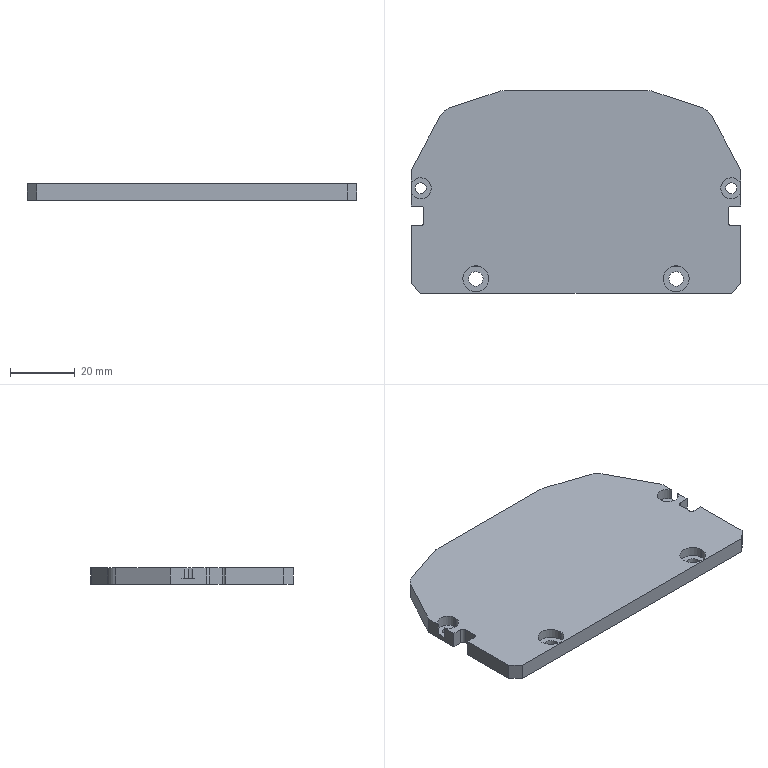Part | SolidWorks | features BaseBody 1 | 1 solid | 47 faces | box 102 x 62.7 x 5 mm | volume 28999 mm3 | plane 24 | cylinder 23 | commonest cylinder face diameters 2 x4 3.4 x4 4.5 x4 8 x4 10 x4 6.5 x3
STEP:
#1=CARTESIAN_POINT('',(20.084,242.618,0.));
#2=VERTEX_POINT('',#1);
#3=CARTESIAN_POINT('',(23.484,242.618,0.));
#4=VERTEX_POINT('',#3);
#5=CARTESIAN_POINT('',(21.784,242.618,0.));
#6=DIRECTION('',(0.,0.,1.));
#7=DIRECTION('',(1.,0.,0.));
#8=AXIS2_PLACEMENT_3D('',#5,#6,#7);
#9=CIRCLE('',#8,1.7);
#10=EDGE_CURVE('',#2,#4,#9,.T.);
#11=ORIENTED_EDGE('',*,*,#10,.F.);
#12=CARTESIAN_POINT('',(20.084,242.618,1.6));
#13=VERTEX_POINT('',#12);
#14=CARTESIAN_POINT('',(20.084,242.618,5.));
#15=DIRECTION('',(0.,0.,1.));
#16=VECTOR('',#15,1000.);
#17=LINE('',#14,#16);
#18=EDGE_CURVE('',#2,#13,#17,.T.);
#19=ORIENTED_EDGE('',*,*,#18,.T.);
#20=CARTESIAN_POINT('',(23.484,242.618,1.6));
#21=VERTEX_POINT('',#20);
#22=CARTESIAN_POINT('',(21.784,242.618,1.6));
#23=DIRECTION('',(0.,0.,-1.));
#24=DIRECTION('',(1.,0.,0.));
#25=AXIS2_PLACEMENT_3D('',#22,#23,#24);
#26=CIRCLE('',#25,1.7);
#27=EDGE_CURVE('',#21,#13,#26,.T.);
#28=ORIENTED_EDGE('',*,*,#27,.F.);
#29=CARTESIAN_POINT('',(23.484,242.618,5.));
#30=DIRECTION('',(0.,0.,1.));
#31=VECTOR('',#30,1000.);
#32=LINE('',#29,#31);
#33=EDGE_CURVE('',#4,#21,#32,.T.);
#34=ORIENTED_EDGE('',*,*,#33,.F.);
#35=EDGE_LOOP('',(#11,#19,#28,#34));
#36=FACE_OUTER_BOUND('',#35,.T.);
#37=CARTESIAN_POINT('',(21.784,242.618,5.));
#38=DIRECTION('',(0.,0.,1.));
#39=DIRECTION('',(1.,0.,0.));
#40=AXIS2_PLACEMENT_3D('',#37,#38,#39);
#41=CYLINDRICAL_SURFACE('',#40,1.7);
#42=ADVANCED_FACE('',(#36),#41,.F.);
#43=CARTESIAN_POINT('',(-59.466,214.618,0.));
#44=VERTEX_POINT('',#43);
#45=CARTESIAN_POINT('',(-54.966,214.618,0.));
#46=VERTEX_POINT('',#45);
#47=CARTESIAN_POINT('',(-57.216,214.618,0.));
#48=DIRECTION('',(0.,0.,1.));
#49=DIRECTION('',(1.,0.,0.));
#50=AXIS2_PLACEMENT_3D('',#47,#48,#49);
#51=CIRCLE('',#50,2.25);
#52=EDGE_CURVE('',#44,#46,#51,.T.);
#53=ORIENTED_EDGE('',*,*,#52,.F.);
#54=CARTESIAN_POINT('',(-59.466,214.618,2.));
#55=VERTEX_POINT('',#54);
#56=CARTESIAN_POINT('',(-59.466,214.618,5.));
#57=DIRECTION('',(0.,0.,1.));
#58=VECTOR('',#57,1000.);
#59=LINE('',#56,#58);
#60=EDGE_CURVE('',#44,#55,#59,.T.);
#61=ORIENTED_EDGE('',*,*,#60,.T.);
#62=CARTESIAN_POINT('',(-54.966,214.618,2.));
#63=VERTEX_POINT('',#62);
#64=CARTESIAN_POINT('',(-57.216,214.618,2.));
#65=DIRECTION('',(0.,0.,-1.));
#66=DIRECTION('',(1.,0.,0.));
#67=AXIS2_PLACEMENT_3D('',#64,#65,#66);
#68=CIRCLE('',#67,2.25);
#69=EDGE_CURVE('',#63,#55,#68,.T.);
#70=ORIENTED_EDGE('',*,*,#69,.F.);
#71=CARTESIAN_POINT('',(-54.966,214.618,5.));
#72=DIRECTION('',(0.,0.,1.));
#73=VECTOR('',#72,1000.);
#74=LINE('',#71,#73);
#75=EDGE_CURVE('',#46,#63,#74,.T.);
#76=ORIENTED_EDGE('',*,*,#75,.F.);
#77=EDGE_LOOP('',(#53,#61,#70,#76));
#78=FACE_OUTER_BOUND('',#77,.T.);
#79=CARTESIAN_POINT('',(-57.216,214.618,5.));
#80=DIRECTION('',(0.,0.,1.));
#81=DIRECTION('',(1.,0.,0.));
#82=AXIS2_PLACEMENT_3D('',#79,#80,#81);
#83=CYLINDRICAL_SURFACE('',#82,2.25);
#84=ADVANCED_FACE('',(#78),#83,.F.);
#85=CARTESIAN_POINT('',(2.534,214.618,0.));
#86=VERTEX_POINT('',#85);
#87=CARTESIAN_POINT('',(7.034,214.618,0.));
#88=VERTEX_POINT('',#87);
#89=CARTESIAN_POINT('',(4.784,214.618,0.));
#90=DIRECTION('',(0.,0.,1.));
#91=DIRECTION('',(1.,0.,0.));
#92=AXIS2_PLACEMENT_3D('',#89,#90,#91);
#93=CIRCLE('',#92,2.25);
#94=EDGE_CURVE('',#86,#88,#93,.T.);
#95=ORIENTED_EDGE('',*,*,#94,.F.);
#96=CARTESIAN_POINT('',(2.534,214.618,2.));
#97=VERTEX_POINT('',#96);
#98=CARTESIAN_POINT('',(2.534,214.618,5.));
#99=DIRECTION('',(0.,0.,1.));
#100=VECTOR('',#99,1000.);
#101=LINE('',#98,#100);
#102=EDGE_CURVE('',#86,#97,#101,.T.);
#103=ORIENTED_EDGE('',*,*,#102,.T.);
#104=CARTESIAN_POINT('',(7.034,214.618,2.));
#105=VERTEX_POINT('',#104);
#106=CARTESIAN_POINT('',(4.784,214.618,2.));
#107=DIRECTION('',(0.,0.,-1.));
#108=DIRECTION('',(1.,0.,0.));
#109=AXIS2_PLACEMENT_3D('',#106,#107,#108);
#110=CIRCLE('',#109,2.25);
#111=EDGE_CURVE('',#105,#97,#110,.T.);
#112=ORIENTED_EDGE('',*,*,#111,.F.);
#113=CARTESIAN_POINT('',(7.034,214.618,5.));
#114=DIRECTION('',(0.,0.,1.));
#115=VECTOR('',#114,1000.);
#116=LINE('',#113,#115);
#117=EDGE_CURVE('',#88,#105,#116,.T.);
#118=ORIENTED_EDGE('',*,*,#117,.F.);
#119=EDGE_LOOP('',(#95,#103,#112,#118));
#120=FACE_OUTER_BOUND('',#119,.T.);
#121=CARTESIAN_POINT('',(4.784,214.618,5.));
#122=DIRECTION('',(0.,0.,1.));
#123=DIRECTION('',(1.,0.,0.));
#124=AXIS2_PLACEMENT_3D('',#121,#122,#123);
#125=CYLINDRICAL_SURFACE('',#124,2.25);
#126=ADVANCED_FACE('',(#120),#125,.F.);
#127=CARTESIAN_POINT('',(-75.916,242.618,0.));
#128=VERTEX_POINT('',#127);
#129=CARTESIAN_POINT('',(-72.516,242.618,0.));
#130=VERTEX_POINT('',#129);
#131=CARTESIAN_POINT('',(-74.216,242.618,0.));
#132=DIRECTION('',(0.,0.,1.));
#133=DIRECTION('',(1.,0.,0.));
#134=AXIS2_PLACEMENT_3D('',#131,#132,#133);
#135=CIRCLE('',#134,1.7);
#136=EDGE_CURVE('',#128,#130,#135,.T.);
#137=ORIENTED_EDGE('',*,*,#136,.F.);
#138=CARTESIAN_POINT('',(-75.916,242.618,1.6));
#139=VERTEX_POINT('',#138);
#140=CARTESIAN_POINT('',(-75.916,242.618,5.));
#141=DIRECTION('',(0.,0.,1.));
#142=VECTOR('',#141,1000.);
#143=LINE('',#140,#142);
#144=EDGE_CURVE('',#128,#139,#143,.T.);
#145=ORIENTED_EDGE('',*,*,#144,.T.);
#146=CARTESIAN_POINT('',(-72.516,242.618,1.6));
#147=VERTEX_POINT('',#146);
#148=CARTESIAN_POINT('',(-74.216,242.618,1.6));
#149=DIRECTION('',(0.,0.,-1.));
#150=DIRECTION('',(1.,0.,0.));
#151=AXIS2_PLACEMENT_3D('',#148,#149,#150);
#152=CIRCLE('',#151,1.7);
#153=EDGE_CURVE('',#147,#139,#152,.T.);
#154=ORIENTED_EDGE('',*,*,#153,.F.);
#155=CARTESIAN_POINT('',(-72.516,242.618,5.));
#156=DIRECTION('',(0.,0.,1.));
#157=VECTOR('',#156,1000.);
#158=LINE('',#155,#157);
#159=EDGE_CURVE('',#130,#147,#158,.T.);
#160=ORIENTED_EDGE('',*,*,#159,.F.);
#161=EDGE_LOOP('',(#137,#145,#154,#160));
#162=FACE_OUTER_BOUND('',#161,.T.);
#163=CARTESIAN_POINT('',(-74.216,242.618,5.));
#164=DIRECTION('',(0.,0.,1.));
#165=DIRECTION('',(1.,0.,0.));
#166=AXIS2_PLACEMENT_3D('',#163,#164,#165);
#167=CYLINDRICAL_SURFACE('',#166,1.7);
#168=ADVANCED_FACE('',(#162),#167,.F.);
#169=CARTESIAN_POINT('',(-77.216,243.868,1.6));
#170=VERTEX_POINT('',#169);
#171=CARTESIAN_POINT('',(-70.966,242.618,1.6));
#172=VERTEX_POINT('',#171);
#173=CARTESIAN_POINT('',(-74.216,242.618,1.6));
#174=DIRECTION('',(0.,0.,-1.));
#175=DIRECTION('',(1.,0.,0.));
#176=AXIS2_PLACEMENT_3D('',#173,#174,#175);
#177=CIRCLE('',#176,3.25);
#178=EDGE_CURVE('',#170,#172,#177,.T.);
#179=ORIENTED_EDGE('',*,*,#178,.T.);
#180=CARTESIAN_POINT('',(-70.966,242.618,5.));
#181=VERTEX_POINT('',#180);
#182=CARTESIAN_POINT('',(-70.966,242.618,5.));
#183=DIRECTION('',(0.,0.,1.));
#184=VECTOR('',#183,1000.);
#185=LINE('',#182,#184);
#186=EDGE_CURVE('',#172,#181,#185,.T.);
#187=ORIENTED_EDGE('',*,*,#186,.T.);
#188=CARTESIAN_POINT('',(-77.216,243.868,5.));
#189=VERTEX_POINT('',#188);
#190=CARTESIAN_POINT('',(-74.216,242.618,5.));
#191=DIRECTION('',(0.,0.,1.));
#192=DIRECTION('',(1.,0.,0.));
#193=AXIS2_PLACEMENT_3D('',#190,#191,#192);
#194=CIRCLE('',#193,3.25);
#195=EDGE_CURVE('',#181,#189,#194,.T.);
#196=ORIENTED_EDGE('',*,*,#195,.T.);
#197=CARTESIAN_POINT('',(-77.216,243.868,5.));
#198=DIRECTION('',(0.,0.,-1.));
#199=VECTOR('',#198,1000.);
#200=LINE('',#197,#199);
#201=EDGE_CURVE('',#189,#170,#200,.T.);
#202=ORIENTED_EDGE('',*,*,#201,.T.);
#203=EDGE_LOOP('',(#179,#187,#196,#202));
#204=FACE_OUTER_BOUND('',#203,.T.);
#205=CARTESIAN_POINT('',(-74.216,242.618,5.));
#206=DIRECTION('',(0.,0.,1.));
#207=DIRECTION('',(1.,0.,0.));
#208=AXIS2_PLACEMENT_3D('',#205,#206,#207);
#209=CYLINDRICAL_SURFACE('',#208,3.25);
#210=ADVANCED_FACE('',(#204),#209,.F.);
#211=CARTESIAN_POINT('',(-53.216,214.618,2.));
#212=VERTEX_POINT('',#211);
#213=CARTESIAN_POINT('',(-61.216,214.618,2.));
#214=VERTEX_POINT('',#213);
#215=CARTESIAN_POINT('',(-57.216,214.618,2.));
#216=DIRECTION('',(0.,0.,-1.));
#217=DIRECTION('',(1.,0.,0.));
#218=AXIS2_PLACEMENT_3D('',#215,#216,#217);
#219=CIRCLE('',#218,4.);
#220=EDGE_CURVE('',#212,#214,#219,.T.);
#221=ORIENTED_EDGE('',*,*,#220,.T.);
#222=CARTESIAN_POINT('',(-61.216,214.618,5.));
#223=VERTEX_POINT('',#222);
#224=CARTESIAN_POINT('',(-61.216,214.618,5.));
#225=DIRECTION('',(0.,0.,1.));
#226=VECTOR('',#225,1000.);
#227=LINE('',#224,#226);
#228=EDGE_CURVE('',#214,#223,#227,.T.);
#229=ORIENTED_EDGE('',*,*,#228,.T.);
#230=CARTESIAN_POINT('',(-53.216,214.618,5.));
#231=VERTEX_POINT('',#230);
#232=CARTESIAN_POINT('',(-57.216,214.618,5.));
#233=DIRECTION('',(0.,0.,1.));
#234=DIRECTION('',(1.,0.,0.));
#235=AXIS2_PLACEMENT_3D('',#232,#233,#234);
#236=CIRCLE('',#235,4.);
#237=EDGE_CURVE('',#223,#231,#236,.T.);
#238=ORIENTED_EDGE('',*,*,#237,.T.);
#239=CARTESIAN_POINT('',(-53.216,214.618,5.));
#240=DIRECTION('',(0.,0.,1.));
#241=VECTOR('',#240,1000.);
#242=LINE('',#239,#241);
#243=EDGE_CURVE('',#212,#231,#242,.T.);
#244=ORIENTED_EDGE('',*,*,#243,.F.);
#245=EDGE_LOOP('',(#221,#229,#238,#244));
#246=FACE_OUTER_BOUND('',#245,.T.);
#247=CARTESIAN_POINT('',(-57.216,214.618,5.));
#248=DIRECTION('',(0.,0.,1.));
#249=DIRECTION('',(1.,0.,0.));
#250=AXIS2_PLACEMENT_3D('',#247,#248,#249);
#251=CYLINDRICAL_SURFACE('',#250,4.);
#252=ADVANCED_FACE('',(#246),#251,.F.);
#253=CARTESIAN_POINT('',(8.784,214.618,2.));
#254=VERTEX_POINT('',#253);
#255=CARTESIAN_POINT('',(0.784,214.618,2.));
#256=VERTEX_POINT('',#255);
#257=CARTESIAN_POINT('',(4.784,214.618,2.));
#258=DIRECTION('',(0.,0.,-1.));
#259=DIRECTION('',(1.,0.,0.));
#260=AXIS2_PLACEMENT_3D('',#257,#258,#259);
#261=CIRCLE('',#260,4.);
#262=EDGE_CURVE('',#254,#256,#261,.T.);
#263=ORIENTED_EDGE('',*,*,#262,.T.);
#264=CARTESIAN_POINT('',(0.784,214.618,5.));
#265=VERTEX_POINT('',#264);
#266=CARTESIAN_POINT('',(0.784,214.618,5.));
#267=DIRECTION('',(0.,0.,1.));
#268=VECTOR('',#267,1000.);
#269=LINE('',#266,#268);
#270=EDGE_CURVE('',#256,#265,#269,.T.);
#271=ORIENTED_EDGE('',*,*,#270,.T.);
#272=CARTESIAN_POINT('',(8.784,214.618,5.));
#273=VERTEX_POINT('',#272);
#274=CARTESIAN_POINT('',(4.784,214.618,5.));
#275=DIRECTION('',(0.,0.,1.));
#276=DIRECTION('',(1.,0.,0.));
#277=AXIS2_PLACEMENT_3D('',#274,#275,#276);
#278=CIRCLE('',#277,4.);
#279=EDGE_CURVE('',#265,#273,#278,.T.);
#280=ORIENTED_EDGE('',*,*,#279,.T.);
#281=CARTESIAN_POINT('',(8.784,214.618,5.));
#282=DIRECTION('',(0.,0.,1.));
#283=VECTOR('',#282,1000.);
#284=LINE('',#281,#283);
#285=EDGE_CURVE('',#254,#273,#284,.T.);
#286=ORIENTED_EDGE('',*,*,#285,.F.);
#287=EDGE_LOOP('',(#263,#271,#280,#286));
#288=FACE_OUTER_BOUND('',#287,.T.);
#289=CARTESIAN_POINT('',(4.784,214.618,5.));
#290=DIRECTION('',(0.,0.,1.));
#291=DIRECTION('',(1.,0.,0.));
#292=AXIS2_PLACEMENT_3D('',#289,#290,#291);
#293=CYLINDRICAL_SURFACE('',#292,4.);
#294=ADVANCED_FACE('',(#288),#293,.F.);
#295=CARTESIAN_POINT('',(21.784,242.618,0.));
#296=DIRECTION('',(0.,0.,1.));
#297=DIRECTION('',(1.,0.,0.));
#298=AXIS2_PLACEMENT_3D('',#295,#296,#297);
#299=CIRCLE('',#298,1.7);
#300=EDGE_CURVE('',#4,#2,#299,.T.);
#301=ORIENTED_EDGE('',*,*,#300,.T.);
#302=ORIENTED_EDGE('',*,*,#10,.T.);
#303=EDGE_LOOP('',(#301,#302));
#304=FACE_BOUND('',#303,.T.);
#305=CARTESIAN_POINT('',(-57.216,214.618,0.));
#306=DIRECTION('',(0.,0.,1.));
#307=DIRECTION('',(1.,0.,0.));
#308=AXIS2_PLACEMENT_3D('',#305,#306,#307);
#309=CIRCLE('',#308,2.25);
#310=EDGE_CURVE('',#46,#44,#309,.T.);
#311=ORIENTED_EDGE('',*,*,#310,.T.);
#312=ORIENTED_EDGE('',*,*,#52,.T.);
#313=EDGE_LOOP('',(#311,#312));
#314=FACE_BOUND('',#313,.T.);
#315=CARTESIAN_POINT('',(4.784,214.618,0.));
#316=DIRECTION('',(0.,0.,1.));
#317=DIRECTION('',(1.,0.,0.));
#318=AXIS2_PLACEMENT_3D('',#315,#316,#317);
#319=CIRCLE('',#318,2.25);
#320=EDGE_CURVE('',#88,#86,#319,.T.);
#321=ORIENTED_EDGE('',*,*,#320,.T.);
#322=ORIENTED_EDGE('',*,*,#94,.T.);
#323=EDGE_LOOP('',(#321,#322));
#324=FACE_BOUND('',#323,.T.);
#325=CARTESIAN_POINT('',(-74.216,242.618,0.));
#326=DIRECTION('',(0.,0.,1.));
#327=DIRECTION('',(1.,0.,0.));
#328=AXIS2_PLACEMENT_3D('',#325,#326,#327);
#329=CIRCLE('',#328,1.7);
#330=EDGE_CURVE('',#130,#128,#329,.T.);
#331=ORIENTED_EDGE('',*,*,#330,.T.);
#332=ORIENTED_EDGE('',*,*,#136,.T.);
#333=EDGE_LOOP('',(#331,#332));
#334=FACE_BOUND('',#333,.T.);
#335=CARTESIAN_POINT('',(20.784,236.118,0.));
#336=VERTEX_POINT('',#335);
#337=CARTESIAN_POINT('',(20.784,232.118,0.));
#338=VERTEX_POINT('',#337);
#339=CARTESIAN_POINT('',(20.784,0.,0.));
#340=DIRECTION('',(0.,-1.,0.));
#341=VECTOR('',#340,1000.);
#342=LINE('',#339,#341);
#343=EDGE_CURVE('',#336,#338,#342,.T.);
#344=ORIENTED_EDGE('',*,*,#343,.T.);
#345=CARTESIAN_POINT('',(21.784,231.118,0.));
#346=VERTEX_POINT('',#345);
#347=CARTESIAN_POINT('',(21.784,232.118,0.));
#348=DIRECTION('',(0.,0.,1.));
#349=DIRECTION('',(-1.,0.,0.));
#350=AXIS2_PLACEMENT_3D('',#347,#348,#349);
#351=CIRCLE('',#350,1.);
#352=EDGE_CURVE('',#338,#346,#351,.T.);
#353=ORIENTED_EDGE('',*,*,#352,.T.);
#354=CARTESIAN_POINT('',(24.784,231.118,0.));
#355=VERTEX_POINT('',#354);
#356=CARTESIAN_POINT('',(0.,231.118,0.));
#357=DIRECTION('',(1.,0.,0.));
#358=VECTOR('',#357,1000.);
#359=LINE('',#356,#358);
#360=EDGE_CURVE('',#346,#355,#359,.T.);
#361=ORIENTED_EDGE('',*,*,#360,.T.);
#362=CARTESIAN_POINT('',(24.784,213.118,0.));
#363=VERTEX_POINT('',#362);
#364=CARTESIAN_POINT('',(24.784,0.,0.));
#365=DIRECTION('',(0.,-1.,0.));
#366=VECTOR('',#365,1000.);
#367=LINE('',#364,#366);
#368=EDGE_CURVE('',#355,#363,#367,.T.);
#369=ORIENTED_EDGE('',*,*,#368,.T.);
#370=CARTESIAN_POINT('',(21.784,210.118,0.));
#371=VERTEX_POINT('',#370);
#372=CARTESIAN_POINT('',(24.784,213.118,0.));
#373=DIRECTION('',(-0.7071,-0.7071,0.));
#374=VECTOR('',#373,1000.);
#375=LINE('',#372,#374);
#376=EDGE_CURVE('',#363,#371,#375,.T.);
#377=ORIENTED_EDGE('',*,*,#376,.T.);
#378=CARTESIAN_POINT('',(-74.216,210.118,0.));
#379=VERTEX_POINT('',#378);
#380=CARTESIAN_POINT('',(0.,210.118,0.));
#381=DIRECTION('',(-1.,0.,0.));
#382=VECTOR('',#381,1000.);
#383=LINE('',#380,#382);
#384=EDGE_CURVE('',#371,#379,#383,.T.);
#385=ORIENTED_EDGE('',*,*,#384,.T.);
#386=CARTESIAN_POINT('',(-77.216,213.118,0.));
#387=VERTEX_POINT('',#386);
#388=CARTESIAN_POINT('',(-74.216,210.118,0.));
#389=DIRECTION('',(-0.7071,0.7071,0.));
#390=VECTOR('',#389,1000.);
#391=LINE('',#388,#390);
#392=EDGE_CURVE('',#379,#387,#391,.T.);
#393=ORIENTED_EDGE('',*,*,#392,.T.);
#394=CARTESIAN_POINT('',(-77.216,231.118,0.));
#395=VERTEX_POINT('',#394);
#396=CARTESIAN_POINT('',(-77.216,0.,0.));
#397=DIRECTION('',(0.,1.,0.));
#398=VECTOR('',#397,1000.);
#399=LINE('',#396,#398);
#400=EDGE_CURVE('',#387,#395,#399,.T.);
#401=ORIENTED_EDGE('',*,*,#400,.T.);
#402=CARTESIAN_POINT('',(-74.216,231.118,0.));
#403=VERTEX_POINT('',#402);
#404=CARTESIAN_POINT('',(0.,231.118,0.));
#405=DIRECTION('',(1.,0.,0.));
#406=VECTOR('',#405,1000.);
#407=LINE('',#404,#406);
#408=EDGE_CURVE('',#395,#403,#407,.T.);
#409=ORIENTED_EDGE('',*,*,#408,.T.);
#410=CARTESIAN_POINT('',(-73.216,232.118,0.));
#411=VERTEX_POINT('',#410);
#412=CARTESIAN_POINT('',(-74.216,232.118,0.));
#413=DIRECTION('',(0.,0.,1.));
#414=DIRECTION('',(-1.,0.,0.));
#415=AXIS2_PLACEMENT_3D('',#412,#413,#414);
#416=CIRCLE('',#415,1.);
#417=EDGE_CURVE('',#403,#411,#416,.T.);
#418=ORIENTED_EDGE('',*,*,#417,.T.);
#419=CARTESIAN_POINT('',(-73.216,236.118,0.));
#420=VERTEX_POINT('',#419);
#421=CARTESIAN_POINT('',(-73.216,0.,0.));
#422=DIRECTION('',(0.,1.,0.));
#423=VECTOR('',#422,1000.);
#424=LINE('',#421,#423);
#425=EDGE_CURVE('',#411,#420,#424,.T.);
#426=ORIENTED_EDGE('',*,*,#425,.T.);
#427=CARTESIAN_POINT('',(-74.216,237.118,0.));
#428=VERTEX_POINT('',#427);
#429=CARTESIAN_POINT('',(-74.216,236.118,0.));
#430=DIRECTION('',(0.,0.,1.));
#431=DIRECTION('',(-1.,0.,0.));
#432=AXIS2_PLACEMENT_3D('',#429,#430,#431);
#433=CIRCLE('',#432,1.);
#434=EDGE_CURVE('',#420,#428,#433,.T.);
#435=ORIENTED_EDGE('',*,*,#434,.T.);
#436=CARTESIAN_POINT('',(-77.216,237.118,0.));
#437=VERTEX_POINT('',#436);
#438=CARTESIAN_POINT('',(0.,237.118,0.));
#439=DIRECTION('',(-1.,0.,0.));
#440=VECTOR('',#439,1000.);
#441=LINE('',#438,#440);
#442=EDGE_CURVE('',#428,#437,#441,.T.);
#443=ORIENTED_EDGE('',*,*,#442,.T.);
#444=CARTESIAN_POINT('',(-77.216,248.118,0.));
#445=VERTEX_POINT('',#444);
#446=CARTESIAN_POINT('',(-77.216,0.,0.));
#447=DIRECTION('',(0.,1.,0.));
#448=VECTOR('',#447,1000.);
#449=LINE('',#446,#448);
#450=EDGE_CURVE('',#437,#445,#449,.T.);
#451=ORIENTED_EDGE('',*,*,#450,.T.);
#452=CARTESIAN_POINT('',(-68.155,265.062,0.));
#453=VERTEX_POINT('',#452);
#454=CARTESIAN_POINT('',(-77.216,248.118,0.));
#455=DIRECTION('',(0.4716,0.8818,0.));
#456=VECTOR('',#455,1000.);
#457=LINE('',#454,#456);
#458=EDGE_CURVE('',#445,#453,#457,.T.);
#459=ORIENTED_EDGE('',*,*,#458,.T.);
#460=CARTESIAN_POINT('',(-65.327,267.447,0.));
#461=VERTEX_POINT('',#460);
#462=CARTESIAN_POINT('',(-63.746,262.704,0.));
#463=DIRECTION('',(0.,0.,-1.));
#464=DIRECTION('',(-1.,0.,0.));
#465=AXIS2_PLACEMENT_3D('',#462,#463,#464);
#466=CIRCLE('',#465,5.);
#467=EDGE_CURVE('',#453,#461,#466,.T.);
#468=ORIENTED_EDGE('',*,*,#467,.T.);
#469=CARTESIAN_POINT('',(-49.986,272.561,0.));
#470=VERTEX_POINT('',#469);
#471=CARTESIAN_POINT('',(-65.327,267.447,0.));
#472=DIRECTION('',(0.9487,0.3162,0.));
#473=VECTOR('',#472,1000.);
#474=LINE('',#471,#473);
#475=EDGE_CURVE('',#461,#470,#474,.T.);
#476=ORIENTED_EDGE('',*,*,#475,.T.);
#477=CARTESIAN_POINT('',(-48.405,272.818,0.));
#478=VERTEX_POINT('',#477);
#479=CARTESIAN_POINT('',(-48.405,267.818,0.));
#480=DIRECTION('',(0.,0.,-1.));
#481=DIRECTION('',(-1.,0.,0.));
#482=AXIS2_PLACEMENT_3D('',#479,#480,#481);
#483=CIRCLE('',#482,5.);
#484=EDGE_CURVE('',#470,#478,#483,.T.);
#485=ORIENTED_EDGE('',*,*,#484,.T.);
#486=CARTESIAN_POINT('',(-4.027,272.818,0.));
#487=VERTEX_POINT('',#486);
#488=CARTESIAN_POINT('',(0.,272.818,0.));
#489=DIRECTION('',(1.,0.,0.));
#490=VECTOR('',#489,1000.);
#491=LINE('',#488,#490);
#492=EDGE_CURVE('',#478,#487,#491,.T.);
#493=ORIENTED_EDGE('',*,*,#492,.T.);
#494=CARTESIAN_POINT('',(-2.446,272.561,0.));
#495=VERTEX_POINT('',#494);
#496=CARTESIAN_POINT('',(-4.027,267.818,0.));
#497=DIRECTION('',(0.,0.,-1.));
#498=DIRECTION('',(-1.,0.,0.));
#499=AXIS2_PLACEMENT_3D('',#496,#497,#498);
#500=CIRCLE('',#499,5.);
#501=EDGE_CURVE('',#487,#495,#500,.T.);
#502=ORIENTED_EDGE('',*,*,#501,.T.);
#503=CARTESIAN_POINT('',(12.895,267.447,0.));
#504=VERTEX_POINT('',#503);
#505=CARTESIAN_POINT('',(-2.446,272.561,0.));
#506=DIRECTION('',(0.9487,-0.3162,0.));
#507=VECTOR('',#506,1000.);
#508=LINE('',#505,#507);
#509=EDGE_CURVE('',#495,#504,#508,.T.);
#510=ORIENTED_EDGE('',*,*,#509,.T.);
#511=CARTESIAN_POINT('',(15.723,265.062,0.));
#512=VERTEX_POINT('',#511);
#513=CARTESIAN_POINT('',(11.314,262.704,0.));
#514=DIRECTION('',(0.,0.,-1.));
#515=DIRECTION('',(-1.,0.,0.));
#516=AXIS2_PLACEMENT_3D('',#513,#514,#515);
#517=CIRCLE('',#516,5.);
#518=EDGE_CURVE('',#504,#512,#517,.T.);
#519=ORIENTED_EDGE('',*,*,#518,.T.);
#520=CARTESIAN_POINT('',(24.784,248.118,0.));
#521=VERTEX_POINT('',#520);
#522=CARTESIAN_POINT('',(15.723,265.062,0.));
#523=DIRECTION('',(0.4716,-0.8818,0.));
#524=VECTOR('',#523,1000.);
#525=LINE('',#522,#524);
#526=EDGE_CURVE('',#512,#521,#525,.T.);
#527=ORIENTED_EDGE('',*,*,#526,.T.);
#528=CARTESIAN_POINT('',(24.784,237.118,0.));
#529=VERTEX_POINT('',#528);
#530=CARTESIAN_POINT('',(24.784,0.,0.));
#531=DIRECTION('',(0.,-1.,0.));
#532=VECTOR('',#531,1000.);
#533=LINE('',#530,#532);
#534=EDGE_CURVE('',#521,#529,#533,.T.);
#535=ORIENTED_EDGE('',*,*,#534,.T.);
#536=CARTESIAN_POINT('',(21.784,237.118,0.));
#537=VERTEX_POINT('',#536);
#538=CARTESIAN_POINT('',(0.,237.118,0.));
#539=DIRECTION('',(-1.,0.,0.));
#540=VECTOR('',#539,1000.);
#541=LINE('',#538,#540);
#542=EDGE_CURVE('',#529,#537,#541,.T.);
#543=ORIENTED_EDGE('',*,*,#542,.T.);
#544=CARTESIAN_POINT('',(21.784,236.118,0.));
#545=DIRECTION('',(0.,0.,1.));
#546=DIRECTION('',(-1.,0.,0.));
#547=AXIS2_PLACEMENT_3D('',#544,#545,#546);
#548=CIRCLE('',#547,1.);
#549=EDGE_CURVE('',#537,#336,#548,.T.);
#550=ORIENTED_EDGE('',*,*,#549,.T.);
#551=EDGE_LOOP('',(#344,#353,#361,#369,#377,#385,#393,#401,#409,#418,#426,#435,#443,#451,#459,#468,#476,#485,#493,#502,#510,#519,#527,#535,#543,#550));
#552=FACE_OUTER_BOUND('',#551,.T.);
#553=CARTESIAN_POINT('',(0.,0.,0.));
#554=DIRECTION('',(0.,0.,-1.));
#555=DIRECTION('',(-1.,0.,0.));
#556=AXIS2_PLACEMENT_3D('',#553,#554,#555);
#557=PLANE('',#556);
#558=ADVANCED_FACE('',(#304,#314,#324,#334,#552),#557,.T.);
#559=ORIENTED_EDGE('',*,*,#18,.F.);
#560=ORIENTED_EDGE('',*,*,#300,.F.);
#561=ORIENTED_EDGE('',*,*,#33,.T.);
#562=CARTESIAN_POINT('',(21.784,242.618,1.6));
#563=DIRECTION('',(0.,0.,-1.));
#564=DIRECTION('',(1.,0.,0.));
#565=AXIS2_PLACEMENT_3D('',#562,#563,#564);
#566=CIRCLE('',#565,1.7);
#567=EDGE_CURVE('',#13,#21,#566,.T.);
#568=ORIENTED_EDGE('',*,*,#567,.F.);
#569=EDGE_LOOP('',(#559,#560,#561,#568));
#570=FACE_OUTER_BOUND('',#569,.T.);
#571=CARTESIAN_POINT('',(21.784,242.618,5.));
#572=DIRECTION('',(0.,0.,1.));
#573=DIRECTION('',(1.,0.,0.));
#574=AXIS2_PLACEMENT_3D('',#571,#572,#573);
#575=CYLINDRICAL_SURFACE('',#574,1.7);
#576=ADVANCED_FACE('',(#570),#575,.F.);
#577=ORIENTED_EDGE('',*,*,#60,.F.);
#578=ORIENTED_EDGE('',*,*,#310,.F.);
#579=ORIENTED_EDGE('',*,*,#75,.T.);
#580=CARTESIAN_POINT('',(-57.216,214.618,2.));
#581=DIRECTION('',(0.,0.,-1.));
#582=DIRECTION('',(1.,0.,0.));
#583=AXIS2_PLACEMENT_3D('',#580,#581,#582);
#584=CIRCLE('',#583,2.25);
#585=EDGE_CURVE('',#55,#63,#584,.T.);
#586=ORIENTED_EDGE('',*,*,#585,.F.);
#587=EDGE_LOOP('',(#577,#578,#579,#586));
#588=FACE_OUTER_BOUND('',#587,.T.);
#589=CARTESIAN_POINT('',(-57.216,214.618,5.));
#590=DIRECTION('',(0.,0.,1.));
#591=DIRECTION('',(1.,0.,0.));
#592=AXIS2_PLACEMENT_3D('',#589,#590,#591);
#593=CYLINDRICAL_SURFACE('',#592,2.25);
#594=ADVANCED_FACE('',(#588),#593,.F.);
#595=ORIENTED_EDGE('',*,*,#102,.F.);
#596=ORIENTED_EDGE('',*,*,#320,.F.);
#597=ORIENTED_EDGE('',*,*,#117,.T.);
#598=CARTESIAN_POINT('',(4.784,214.618,2.));
#599=DIRECTION('',(0.,0.,-1.));
#600=DIRECTION('',(1.,0.,0.));
#601=AXIS2_PLACEMENT_3D('',#598,#599,#600);
#602=CIRCLE('',#601,2.25);
#603=EDGE_CURVE('',#97,#105,#602,.T.);
#604=ORIENTED_EDGE('',*,*,#603,.F.);
#605=EDGE_LOOP('',(#595,#596,#597,#604));
#606=FACE_OUTER_BOUND('',#605,.T.);
#607=CARTESIAN_POINT('',(4.784,214.618,5.));
#608=DIRECTION('',(0.,0.,1.));
#609=DIRECTION('',(1.,0.,0.));
#610=AXIS2_PLACEMENT_3D('',#607,#608,#609);
#611=CYLINDRICAL_SURFACE('',#610,2.25);
#612=ADVANCED_FACE('',(#606),#611,.F.);
#613=ORIENTED_EDGE('',*,*,#144,.F.);
#614=ORIENTED_EDGE('',*,*,#330,.F.);
#615=ORIENTED_EDGE('',*,*,#159,.T.);
#616=CARTESIAN_POINT('',(-74.216,242.618,1.6));
#617=DIRECTION('',(0.,0.,-1.));
#618=DIRECTION('',(1.,0.,0.));
#619=AXIS2_PLACEMENT_3D('',#616,#617,#618);
#620=CIRCLE('',#619,1.7);
#621=EDGE_CURVE('',#139,#147,#620,.T.);
#622=ORIENTED_EDGE('',*,*,#621,.F.);
#623=EDGE_LOOP('',(#613,#614,#615,#622));
#624=FACE_OUTER_BOUND('',#623,.T.);
#625=CARTESIAN_POINT('',(-74.216,242.618,5.));
#626=DIRECTION('',(0.,0.,1.));
#627=DIRECTION('',(1.,0.,0.));
#628=AXIS2_PLACEMENT_3D('',#625,#626,#627);
#629=CYLINDRICAL_SURFACE('',#628,1.7);
#630=ADVANCED_FACE('',(#624),#629,.F.);
#631=CARTESIAN_POINT('',(20.784,232.118,5.));
#632=VERTEX_POINT('',#631);
#633=CARTESIAN_POINT('',(20.784,232.118,-5.));
#634=DIRECTION('',(0.,0.,-1.));
#635=VECTOR('',#634,1000.);
#636=LINE('',#633,#635);
#637=EDGE_CURVE('',#632,#338,#636,.T.);
#638=ORIENTED_EDGE('',*,*,#637,.F.);
#639=CARTESIAN_POINT('',(21.784,231.118,5.));
#640=VERTEX_POINT('',#639);
#641=CARTESIAN_POINT('',(21.784,232.118,5.));
#642=DIRECTION('',(0.,0.,-1.));
#643=DIRECTION('',(-1.,0.,0.));
#644=AXIS2_PLACEMENT_3D('',#641,#642,#643);
#645=CIRCLE('',#644,1.);
#646=EDGE_CURVE('',#640,#632,#645,.T.);
#647=ORIENTED_EDGE('',*,*,#646,.F.);
#648=CARTESIAN_POINT('',(21.784,231.118,-5.));
#649=DIRECTION('',(0.,0.,1.));
#650=VECTOR('',#649,1000.);
#651=LINE('',#648,#650);
#652=EDGE_CURVE('',#346,#640,#651,.T.);
#653=ORIENTED_EDGE('',*,*,#652,.F.);
#654=ORIENTED_EDGE('',*,*,#352,.F.);
#655=EDGE_LOOP('',(#638,#647,#653,#654));
#656=FACE_OUTER_BOUND('',#655,.T.);
#657=CARTESIAN_POINT('',(21.784,232.118,-5.));
#658=DIRECTION('',(0.,0.,-1.));
#659=DIRECTION('',(-1.,0.,0.));
#660=AXIS2_PLACEMENT_3D('',#657,#658,#659);
#661=CYLINDRICAL_SURFACE('',#660,1.);
#662=ADVANCED_FACE('',(#656),#661,.F.);
#663=ORIENTED_EDGE('',*,*,#637,.T.);
#664=ORIENTED_EDGE('',*,*,#343,.F.);
#665=CARTESIAN_POINT('',(20.784,236.118,5.));
#666=VERTEX_POINT('',#665);
#667=CARTESIAN_POINT('',(20.784,236.118,-5.));
#668=DIRECTION('',(0.,0.,-1.));
#669=VECTOR('',#668,1000.);
#670=LINE('',#667,#669);
#671=EDGE_CURVE('',#666,#336,#670,.T.);
#672=ORIENTED_EDGE('',*,*,#671,.F.);
#673=CARTESIAN_POINT('',(20.784,237.118,5.));
#674=DIRECTION('',(0.,1.,0.));
#675=VECTOR('',#674,1000.);
#676=LINE('',#673,#675);
#677=EDGE_CURVE('',#632,#666,#676,.T.);
#678=ORIENTED_EDGE('',*,*,#677,.F.);
#679=EDGE_LOOP('',(#663,#664,#672,#678));
#680=FACE_OUTER_BOUND('',#679,.T.);
#681=CARTESIAN_POINT('',(20.784,237.118,-5.));
#682=DIRECTION('',(-1.,0.,0.));
#683=DIRECTION('',(0.,0.,1.));
#684=AXIS2_PLACEMENT_3D('',#681,#682,#683);
#685=PLANE('',#684);
#686=ADVANCED_FACE('',(#680),#685,.F.);
#687=CARTESIAN_POINT('',(21.784,237.118,5.));
#688=VERTEX_POINT('',#687);
#689=CARTESIAN_POINT('',(21.784,237.118,-5.));
#690=DIRECTION('',(0.,0.,-1.));
#691=VECTOR('',#690,1000.);
#692=LINE('',#689,#691);
#693=EDGE_CURVE('',#688,#537,#692,.T.);
#694=ORIENTED_EDGE('',*,*,#693,.F.);
#695=CARTESIAN_POINT('',(21.784,236.118,5.));
#696=DIRECTION('',(0.,0.,-1.));
#697=DIRECTION('',(-1.,0.,0.));
#698=AXIS2_PLACEMENT_3D('',#695,#696,#697);
#699=CIRCLE('',#698,1.);
#700=EDGE_CURVE('',#666,#688,#699,.T.);
#701=ORIENTED_EDGE('',*,*,#700,.F.);
#702=ORIENTED_EDGE('',*,*,#671,.T.);
#703=ORIENTED_EDGE('',*,*,#549,.F.);
#704=EDGE_LOOP('',(#694,#701,#702,#703));
#705=FACE_OUTER_BOUND('',#704,.T.);
#706=CARTESIAN_POINT('',(21.784,236.118,-5.));
#707=DIRECTION('',(0.,0.,-1.));
#708=DIRECTION('',(-1.,0.,0.));
#709=AXIS2_PLACEMENT_3D('',#706,#707,#708);
#710=CYLINDRICAL_SURFACE('',#709,1.);
#711=ADVANCED_FACE('',(#705),#710,.F.);
#712=ORIENTED_EDGE('',*,*,#693,.T.);
#713=ORIENTED_EDGE('',*,*,#542,.F.);
#714=CARTESIAN_POINT('',(24.784,237.118,5.));
#715=VERTEX_POINT('',#714);
#716=CARTESIAN_POINT('',(24.784,237.118,-5.));
#717=DIRECTION('',(0.,0.,-1.));
#718=VECTOR('',#717,1000.);
#719=LINE('',#716,#718);
#720=EDGE_CURVE('',#715,#529,#719,.T.);
#721=ORIENTED_EDGE('',*,*,#720,.F.);
#722=CARTESIAN_POINT('',(29.061,237.118,5.));
#723=DIRECTION('',(1.,0.,0.));
#724=VECTOR('',#723,1000.);
#725=LINE('',#722,#724);
#726=EDGE_CURVE('',#688,#715,#725,.T.);
#727=ORIENTED_EDGE('',*,*,#726,.F.);
#728=EDGE_LOOP('',(#712,#713,#721,#727));
#729=FACE_OUTER_BOUND('',#728,.T.);
#730=CARTESIAN_POINT('',(29.061,237.118,-5.));
#731=DIRECTION('',(0.,1.,0.));
#732=DIRECTION('',(0.,0.,1.));
#733=AXIS2_PLACEMENT_3D('',#730,#731,#732);
#734=PLANE('',#733);
#735=ADVANCED_FACE('',(#729),#734,.F.);
#736=ORIENTED_EDGE('',*,*,#720,.T.);
#737=ORIENTED_EDGE('',*,*,#534,.F.);
#738=CARTESIAN_POINT('',(24.784,248.118,5.));
#739=VERTEX_POINT('',#738);
#740=CARTESIAN_POINT('',(24.784,248.118,5.));
#741=DIRECTION('',(0.,0.,-1.));
#742=VECTOR('',#741,1000.);
#743=LINE('',#740,#742);
#744=EDGE_CURVE('',#739,#521,#743,.T.);
#745=ORIENTED_EDGE('',*,*,#744,.F.);
#746=CARTESIAN_POINT('',(24.784,243.868,5.));
#747=VERTEX_POINT('',#746);
#748=CARTESIAN_POINT('',(24.784,248.118,5.));
#749=DIRECTION('',(0.,1.,0.));
#750=VECTOR('',#749,1000.);
#751=LINE('',#748,#750);
#752=EDGE_CURVE('',#747,#739,#751,.T.);
#753=ORIENTED_EDGE('',*,*,#752,.F.);
#754=CARTESIAN_POINT('',(24.784,243.868,1.6));
#755=VERTEX_POINT('',#754);
#756=CARTESIAN_POINT('',(24.784,243.868,5.));
#757=DIRECTION('',(0.,0.,1.));
#758=VECTOR('',#757,1000.);
#759=LINE('',#756,#758);
#760=EDGE_CURVE('',#755,#747,#759,.T.);
#761=ORIENTED_EDGE('',*,*,#760,.F.);
#762=CARTESIAN_POINT('',(24.784,241.368,1.6));
#763=VERTEX_POINT('',#762);
#764=CARTESIAN_POINT('',(24.784,248.118,1.6));
#765=DIRECTION('',(0.,1.,0.));
#766=VECTOR('',#765,1000.);
#767=LINE('',#764,#766);
#768=EDGE_CURVE('',#763,#755,#767,.T.);
#769=ORIENTED_EDGE('',*,*,#768,.F.);
#770=CARTESIAN_POINT('',(24.784,241.368,5.));
#771=VERTEX_POINT('',#770);
#772=CARTESIAN_POINT('',(24.784,241.368,5.));
#773=DIRECTION('',(0.,0.,-1.));
#774=VECTOR('',#773,1000.);
#775=LINE('',#772,#774);
#776=EDGE_CURVE('',#771,#763,#775,.T.);
#777=ORIENTED_EDGE('',*,*,#776,.F.);
#778=CARTESIAN_POINT('',(24.784,248.118,5.));
#779=DIRECTION('',(0.,1.,0.));
#780=VECTOR('',#779,1000.);
#781=LINE('',#778,#780);
#782=EDGE_CURVE('',#715,#771,#781,.T.);
#783=ORIENTED_EDGE('',*,*,#782,.F.);
#784=EDGE_LOOP('',(#736,#737,#745,#753,#761,#769,#777,#783));
#785=FACE_OUTER_BOUND('',#784,.T.);
#786=CARTESIAN_POINT('',(24.784,248.118,5.));
#787=DIRECTION('',(-1.,0.,0.));
#788=DIRECTION('',(0.,-1.,0.));
#789=AXIS2_PLACEMENT_3D('',#786,#787,#788);
#790=PLANE('',#789);
#791=ADVANCED_FACE('',(#785),#790,.F.);
#792=CARTESIAN_POINT('',(15.723,265.062,5.));
#793=VERTEX_POINT('',#792);
#794=CARTESIAN_POINT('',(15.723,265.062,5.));
#795=DIRECTION('',(0.,0.,-1.));
#796=VECTOR('',#795,1000.);
#797=LINE('',#794,#796);
#798=EDGE_CURVE('',#793,#512,#797,.T.);
#799=ORIENTED_EDGE('',*,*,#798,.F.);
#800=CARTESIAN_POINT('',(14.784,266.818,5.));
#801=DIRECTION('',(-0.4716,0.8818,0.));
#802=VECTOR('',#801,1000.);
#803=LINE('',#800,#802);
#804=EDGE_CURVE('',#739,#793,#803,.T.);
#805=ORIENTED_EDGE('',*,*,#804,.F.);
#806=ORIENTED_EDGE('',*,*,#744,.T.);
#807=ORIENTED_EDGE('',*,*,#526,.F.);
#808=EDGE_LOOP('',(#799,#805,#806,#807));
#809=FACE_OUTER_BOUND('',#808,.T.);
#810=CARTESIAN_POINT('',(14.784,266.818,5.));
#811=DIRECTION('',(-0.8818,-0.4716,0.));
#812=DIRECTION('',(0.4716,-0.8818,0.));
#813=AXIS2_PLACEMENT_3D('',#810,#811,#812);
#814=PLANE('',#813);
#815=ADVANCED_FACE('',(#809),#814,.F.);
#816=ORIENTED_EDGE('',*,*,#518,.F.);
#817=CARTESIAN_POINT('',(12.895,267.447,5.));
#818=VERTEX_POINT('',#817);
#819=CARTESIAN_POINT('',(12.895,267.447,5.));
#820=DIRECTION('',(0.,0.,1.));
#821=VECTOR('',#820,1000.);
#822=LINE('',#819,#821);
#823=EDGE_CURVE('',#504,#818,#822,.T.);
#824=ORIENTED_EDGE('',*,*,#823,.T.);
#825=CARTESIAN_POINT('',(11.314,262.704,5.));
#826=DIRECTION('',(0.,0.,-1.));
#827=DIRECTION('',(-1.,0.,0.));
#828=AXIS2_PLACEMENT_3D('',#825,#826,#827);
#829=CIRCLE('',#828,5.);
#830=EDGE_CURVE('',#818,#793,#829,.T.);
#831=ORIENTED_EDGE('',*,*,#830,.T.);
#832=ORIENTED_EDGE('',*,*,#798,.T.);
#833=EDGE_LOOP('',(#816,#824,#831,#832));
#834=FACE_OUTER_BOUND('',#833,.T.);
#835=CARTESIAN_POINT('',(11.314,262.704,5.));
#836=DIRECTION('',(0.,0.,-1.));
#837=DIRECTION('',(-1.,0.,0.));
#838=AXIS2_PLACEMENT_3D('',#835,#836,#837);
#839=CYLINDRICAL_SURFACE('',#838,5.);
#840=ADVANCED_FACE('',(#834),#839,.T.);
#841=ORIENTED_EDGE('',*,*,#823,.F.);
#842=ORIENTED_EDGE('',*,*,#509,.F.);
#843=CARTESIAN_POINT('',(-2.446,272.561,5.));
#844=VERTEX_POINT('',#843);
#845=CARTESIAN_POINT('',(-2.446,272.561,5.));
#846=DIRECTION('',(0.,0.,-1.));
#847=VECTOR('',#846,1000.);
#848=LINE('',#845,#847);
#849=EDGE_CURVE('',#844,#495,#848,.T.);
#850=ORIENTED_EDGE('',*,*,#849,.F.);
#851=CARTESIAN_POINT('',(-3.216,272.818,5.));
#852=DIRECTION('',(-0.9487,0.3162,0.));
#853=VECTOR('',#852,1000.);
#854=LINE('',#851,#853);
#855=EDGE_CURVE('',#818,#844,#854,.T.);
#856=ORIENTED_EDGE('',*,*,#855,.F.);
#857=EDGE_LOOP('',(#841,#842,#850,#856));
#858=FACE_OUTER_BOUND('',#857,.T.);
#859=CARTESIAN_POINT('',(-3.216,272.818,5.));
#860=DIRECTION('',(-0.3162,-0.9487,0.));
#861=DIRECTION('',(0.9487,-0.3162,0.));
#862=AXIS2_PLACEMENT_3D('',#859,#860,#861);
#863=PLANE('',#862);
#864=ADVANCED_FACE('',(#858),#863,.F.);
#865=ORIENTED_EDGE('',*,*,#501,.F.);
#866=CARTESIAN_POINT('',(-4.027,272.818,5.));
#867=VERTEX_POINT('',#866);
#868=CARTESIAN_POINT('',(-4.027,272.818,5.));
#869=DIRECTION('',(0.,0.,1.));
#870=VECTOR('',#869,1000.);
#871=LINE('',#868,#870);
#872=EDGE_CURVE('',#487,#867,#871,.T.);
#873=ORIENTED_EDGE('',*,*,#872,.T.);
#874=CARTESIAN_POINT('',(-4.027,267.818,5.));
#875=DIRECTION('',(0.,0.,-1.));
#876=DIRECTION('',(-1.,0.,0.));
#877=AXIS2_PLACEMENT_3D('',#874,#875,#876);
#878=CIRCLE('',#877,5.);
#879=EDGE_CURVE('',#867,#844,#878,.T.);
#880=ORIENTED_EDGE('',*,*,#879,.T.);
#881=ORIENTED_EDGE('',*,*,#849,.T.);
#882=EDGE_LOOP('',(#865,#873,#880,#881));
#883=FACE_OUTER_BOUND('',#882,.T.);
#884=CARTESIAN_POINT('',(-4.027,267.818,5.));
#885=DIRECTION('',(0.,0.,-1.));
#886=DIRECTION('',(-1.,0.,0.));
#887=AXIS2_PLACEMENT_3D('',#884,#885,#886);
#888=CYLINDRICAL_SURFACE('',#887,5.);
#889=ADVANCED_FACE('',(#883),#888,.T.);
#890=ORIENTED_EDGE('',*,*,#872,.F.);
#891=ORIENTED_EDGE('',*,*,#492,.F.);
#892=CARTESIAN_POINT('',(-48.405,272.818,5.));
#893=VERTEX_POINT('',#892);
#894=CARTESIAN_POINT('',(-48.405,272.818,5.));
#895=DIRECTION('',(0.,0.,-1.));
#896=VECTOR('',#895,1000.);
#897=LINE('',#894,#896);
#898=EDGE_CURVE('',#893,#478,#897,.T.);
#899=ORIENTED_EDGE('',*,*,#898,.F.);
#900=CARTESIAN_POINT('',(-49.216,272.818,5.));
#901=DIRECTION('',(-1.,0.,0.));
#902=VECTOR('',#901,1000.);
#903=LINE('',#900,#902);
#904=EDGE_CURVE('',#867,#893,#903,.T.);
#905=ORIENTED_EDGE('',*,*,#904,.F.);
#906=EDGE_LOOP('',(#890,#891,#899,#905));
#907=FACE_OUTER_BOUND('',#906,.T.);
#908=CARTESIAN_POINT('',(-49.216,272.818,5.));
#909=DIRECTION('',(0.,-1.,0.));
#910=DIRECTION('',(0.,0.,-1.));
#911=AXIS2_PLACEMENT_3D('',#908,#909,#910);
#912=PLANE('',#911);
#913=ADVANCED_FACE('',(#907),#912,.F.);
#914=ORIENTED_EDGE('',*,*,#484,.F.);
#915=CARTESIAN_POINT('',(-49.986,272.561,5.));
#916=VERTEX_POINT('',#915);
#917=CARTESIAN_POINT('',(-49.986,272.561,5.));
#918=DIRECTION('',(0.,0.,1.));
#919=VECTOR('',#918,1000.);
#920=LINE('',#917,#919);
#921=EDGE_CURVE('',#470,#916,#920,.T.);
#922=ORIENTED_EDGE('',*,*,#921,.T.);
#923=CARTESIAN_POINT('',(-48.405,267.818,5.));
#924=DIRECTION('',(0.,0.,-1.));
#925=DIRECTION('',(-1.,0.,0.));
#926=AXIS2_PLACEMENT_3D('',#923,#924,#925);
#927=CIRCLE('',#926,5.);
#928=EDGE_CURVE('',#916,#893,#927,.T.);
#929=ORIENTED_EDGE('',*,*,#928,.T.);
#930=ORIENTED_EDGE('',*,*,#898,.T.);
#931=EDGE_LOOP('',(#914,#922,#929,#930));
#932=FACE_OUTER_BOUND('',#931,.T.);
#933=CARTESIAN_POINT('',(-48.405,267.818,5.));
#934=DIRECTION('',(0.,0.,-1.));
#935=DIRECTION('',(-1.,0.,0.));
#936=AXIS2_PLACEMENT_3D('',#933,#934,#935);
#937=CYLINDRICAL_SURFACE('',#936,5.);
#938=ADVANCED_FACE('',(#932),#937,.T.);
#939=CARTESIAN_POINT('',(-65.327,267.447,5.));
#940=VERTEX_POINT('',#939);
#941=CARTESIAN_POINT('',(-65.327,267.447,5.));
#942=DIRECTION('',(0.,0.,-1.));
#943=VECTOR('',#942,1000.);
#944=LINE('',#941,#943);
#945=EDGE_CURVE('',#940,#461,#944,.T.);
#946=ORIENTED_EDGE('',*,*,#945,.F.);
#947=CARTESIAN_POINT('',(-67.216,266.818,5.));
#948=DIRECTION('',(-0.9487,-0.3162,0.));
#949=VECTOR('',#948,1000.);
#950=LINE('',#947,#949);
#951=EDGE_CURVE('',#916,#940,#950,.T.);
#952=ORIENTED_EDGE('',*,*,#951,.F.);
#953=ORIENTED_EDGE('',*,*,#921,.F.);
#954=ORIENTED_EDGE('',*,*,#475,.F.);
#955=EDGE_LOOP('',(#946,#952,#953,#954));
#956=FACE_OUTER_BOUND('',#955,.T.);
#957=CARTESIAN_POINT('',(-67.216,266.818,5.));
#958=DIRECTION('',(0.3162,-0.9487,0.));
#959=DIRECTION('',(0.9487,0.3162,0.));
#960=AXIS2_PLACEMENT_3D('',#957,#958,#959);
#961=PLANE('',#960);
#962=ADVANCED_FACE('',(#956),#961,.F.);
#963=ORIENTED_EDGE('',*,*,#467,.F.);
#964=CARTESIAN_POINT('',(-68.155,265.062,5.));
#965=VERTEX_POINT('',#964);
#966=CARTESIAN_POINT('',(-68.155,265.062,5.));
#967=DIRECTION('',(0.,0.,1.));
#968=VECTOR('',#967,1000.);
#969=LINE('',#966,#968);
#970=EDGE_CURVE('',#453,#965,#969,.T.);
#971=ORIENTED_EDGE('',*,*,#970,.T.);
#972=CARTESIAN_POINT('',(-63.746,262.704,5.));
#973=DIRECTION('',(0.,0.,-1.));
#974=DIRECTION('',(-1.,0.,0.));
#975=AXIS2_PLACEMENT_3D('',#972,#973,#974);
#976=CIRCLE('',#975,5.);
#977=EDGE_CURVE('',#965,#940,#976,.T.);
#978=ORIENTED_EDGE('',*,*,#977,.T.);
#979=ORIENTED_EDGE('',*,*,#945,.T.);
#980=EDGE_LOOP('',(#963,#971,#978,#979));
#981=FACE_OUTER_BOUND('',#980,.T.);
#982=CARTESIAN_POINT('',(-63.746,262.704,5.));
#983=DIRECTION('',(0.,0.,-1.));
#984=DIRECTION('',(-1.,0.,0.));
#985=AXIS2_PLACEMENT_3D('',#982,#983,#984);
#986=CYLINDRICAL_SURFACE('',#985,5.);
#987=ADVANCED_FACE('',(#981),#986,.T.);
#988=ORIENTED_EDGE('',*,*,#970,.F.);
#989=ORIENTED_EDGE('',*,*,#458,.F.);
#990=CARTESIAN_POINT('',(-77.216,248.118,5.));
#991=VERTEX_POINT('',#990);
#992=CARTESIAN_POINT('',(-77.216,248.118,5.));
#993=DIRECTION('',(0.,0.,-1.));
#994=VECTOR('',#993,1000.);
#995=LINE('',#992,#994);
#996=EDGE_CURVE('',#991,#445,#995,.T.);
#997=ORIENTED_EDGE('',*,*,#996,.F.);
#998=CARTESIAN_POINT('',(-77.216,248.118,5.));
#999=DIRECTION('',(-0.4716,-0.8818,0.));
#1000=VECTOR('',#999,1000.);
#1001=LINE('',#998,#1000);
#1002=EDGE_CURVE('',#965,#991,#1001,.T.);
#1003=ORIENTED_EDGE('',*,*,#1002,.F.);
#1004=EDGE_LOOP('',(#988,#989,#997,#1003));
#1005=FACE_OUTER_BOUND('',#1004,.T.);
#1006=CARTESIAN_POINT('',(-77.216,248.118,5.));
#1007=DIRECTION('',(0.8818,-0.4716,0.));
#1008=DIRECTION('',(0.4716,0.8818,0.));
#1009=AXIS2_PLACEMENT_3D('',#1006,#1007,#1008);
#1010=PLANE('',#1009);
#1011=ADVANCED_FACE('',(#1005),#1010,.F.);
#1012=CARTESIAN_POINT('',(-77.216,237.118,5.));
#1013=VERTEX_POINT('',#1012);
#1014=CARTESIAN_POINT('',(-77.216,237.118,5.));
#1015=DIRECTION('',(0.,0.,-1.));
#1016=VECTOR('',#1015,1000.);
#1017=LINE('',#1014,#1016);
#1018=EDGE_CURVE('',#1013,#437,#1017,.T.);
#1019=ORIENTED_EDGE('',*,*,#1018,.F.);
#1020=CARTESIAN_POINT('',(-77.216,241.368,5.));
#1021=VERTEX_POINT('',#1020);
#1022=CARTESIAN_POINT('',(-77.216,248.118,5.));
#1023=DIRECTION('',(0.,-1.,0.));
#1024=VECTOR('',#1023,1000.);
#1025=LINE('',#1022,#1024);
#1026=EDGE_CURVE('',#1021,#1013,#1025,.T.);
#1027=ORIENTED_EDGE('',*,*,#1026,.F.);
#1028=CARTESIAN_POINT('',(-77.216,241.368,1.6));
#1029=VERTEX_POINT('',#1028);
#1030=CARTESIAN_POINT('',(-77.216,241.368,5.));
#1031=DIRECTION('',(0.,0.,1.));
#1032=VECTOR('',#1031,1000.);
#1033=LINE('',#1030,#1032);
#1034=EDGE_CURVE('',#1029,#1021,#1033,.T.);
#1035=ORIENTED_EDGE('',*,*,#1034,.F.);
#1036=CARTESIAN_POINT('',(-77.216,248.118,1.6));
#1037=DIRECTION('',(0.,-1.,0.));
#1038=VECTOR('',#1037,1000.);
#1039=LINE('',#1036,#1038);
#1040=EDGE_CURVE('',#170,#1029,#1039,.T.);
#1041=ORIENTED_EDGE('',*,*,#1040,.F.);
#1042=ORIENTED_EDGE('',*,*,#201,.F.);
#1043=CARTESIAN_POINT('',(-77.216,248.118,5.));
#1044=DIRECTION('',(0.,-1.,0.));
#1045=VECTOR('',#1044,1000.);
#1046=LINE('',#1043,#1045);
#1047=EDGE_CURVE('',#991,#189,#1046,.T.);
#1048=ORIENTED_EDGE('',*,*,#1047,.F.);
#1049=ORIENTED_EDGE('',*,*,#996,.T.);
#1050=ORIENTED_EDGE('',*,*,#450,.F.);
#1051=EDGE_LOOP('',(#1019,#1027,#1035,#1041,#1042,#1048,#1049,#1050));
#1052=FACE_OUTER_BOUND('',#1051,.T.);
#1053=CARTESIAN_POINT('',(-77.216,248.118,5.));
#1054=DIRECTION('',(1.,0.,0.));
#1055=DIRECTION('',(0.,1.,0.));
#1056=AXIS2_PLACEMENT_3D('',#1053,#1054,#1055);
#1057=PLANE('',#1056);
#1058=ADVANCED_FACE('',(#1052),#1057,.F.);
#1059=CARTESIAN_POINT('',(-74.216,237.118,5.));
#1060=VERTEX_POINT('',#1059);
#1061=CARTESIAN_POINT('',(-74.216,237.118,-5.));
#1062=DIRECTION('',(0.,0.,-1.));
#1063=VECTOR('',#1062,1000.);
#1064=LINE('',#1061,#1063);
#1065=EDGE_CURVE('',#1060,#428,#1064,.T.);
#1066=ORIENTED_EDGE('',*,*,#1065,.F.);
#1067=CARTESIAN_POINT('',(-79.864,237.118,5.));
#1068=DIRECTION('',(1.,0.,0.));
#1069=VECTOR('',#1068,1000.);
#1070=LINE('',#1067,#1069);
#1071=EDGE_CURVE('',#1013,#1060,#1070,.T.);
#1072=ORIENTED_EDGE('',*,*,#1071,.F.);
#1073=ORIENTED_EDGE('',*,*,#1018,.T.);
#1074=ORIENTED_EDGE('',*,*,#442,.F.);
#1075=EDGE_LOOP('',(#1066,#1072,#1073,#1074));
#1076=FACE_OUTER_BOUND('',#1075,.T.);
#1077=CARTESIAN_POINT('',(-79.864,237.118,-5.));
#1078=DIRECTION('',(0.,1.,0.));
#1079=DIRECTION('',(0.,0.,1.));
#1080=AXIS2_PLACEMENT_3D('',#1077,#1078,#1079);
#1081=PLANE('',#1080);
#1082=ADVANCED_FACE('',(#1076),#1081,.F.);
#1083=CARTESIAN_POINT('',(-73.216,236.118,5.));
#1084=VERTEX_POINT('',#1083);
#1085=CARTESIAN_POINT('',(-73.216,236.118,-5.));
#1086=DIRECTION('',(0.,0.,-1.));
#1087=VECTOR('',#1086,1000.);
#1088=LINE('',#1085,#1087);
#1089=EDGE_CURVE('',#1084,#420,#1088,.T.);
#1090=ORIENTED_EDGE('',*,*,#1089,.F.);
#1091=CARTESIAN_POINT('',(-74.216,236.118,5.));
#1092=DIRECTION('',(0.,0.,-1.));
#1093=DIRECTION('',(-1.,0.,0.));
#1094=AXIS2_PLACEMENT_3D('',#1091,#1092,#1093);
#1095=CIRCLE('',#1094,1.);
#1096=EDGE_CURVE('',#1060,#1084,#1095,.T.);
#1097=ORIENTED_EDGE('',*,*,#1096,.F.);
#1098=ORIENTED_EDGE('',*,*,#1065,.T.);
#1099=ORIENTED_EDGE('',*,*,#434,.F.);
#1100=EDGE_LOOP('',(#1090,#1097,#1098,#1099));
#1101=FACE_OUTER_BOUND('',#1100,.T.);
#1102=CARTESIAN_POINT('',(-74.216,236.118,-5.));
#1103=DIRECTION('',(0.,0.,-1.));
#1104=DIRECTION('',(-1.,0.,0.));
#1105=AXIS2_PLACEMENT_3D('',#1102,#1103,#1104);
#1106=CYLINDRICAL_SURFACE('',#1105,1.);
#1107=ADVANCED_FACE('',(#1101),#1106,.F.);
#1108=CARTESIAN_POINT('',(-73.216,232.118,5.));
#1109=VERTEX_POINT('',#1108);
#1110=CARTESIAN_POINT('',(-73.216,232.118,-5.));
#1111=DIRECTION('',(0.,0.,-1.));
#1112=VECTOR('',#1111,1000.);
#1113=LINE('',#1110,#1112);
#1114=EDGE_CURVE('',#1109,#411,#1113,.T.);
#1115=ORIENTED_EDGE('',*,*,#1114,.F.);
#1116=CARTESIAN_POINT('',(-73.216,237.118,5.));
#1117=DIRECTION('',(0.,-1.,0.));
#1118=VECTOR('',#1117,1000.);
#1119=LINE('',#1116,#1118);
#1120=EDGE_CURVE('',#1084,#1109,#1119,.T.);
#1121=ORIENTED_EDGE('',*,*,#1120,.F.);
#1122=ORIENTED_EDGE('',*,*,#1089,.T.);
#1123=ORIENTED_EDGE('',*,*,#425,.F.);
#1124=EDGE_LOOP('',(#1115,#1121,#1122,#1123));
#1125=FACE_OUTER_BOUND('',#1124,.T.);
#1126=CARTESIAN_POINT('',(-73.216,237.118,-5.));
#1127=DIRECTION('',(1.,0.,0.));
#1128=DIRECTION('',(0.,0.,-1.));
#1129=AXIS2_PLACEMENT_3D('',#1126,#1127,#1128);
#1130=PLANE('',#1129);
#1131=ADVANCED_FACE('',(#1125),#1130,.F.);
#1132=CARTESIAN_POINT('',(-74.216,231.118,5.));
#1133=VERTEX_POINT('',#1132);
#1134=CARTESIAN_POINT('',(-74.216,231.118,-5.));
#1135=DIRECTION('',(0.,0.,-1.));
#1136=VECTOR('',#1135,1000.);
#1137=LINE('',#1134,#1136);
#1138=EDGE_CURVE('',#1133,#403,#1137,.T.);
#1139=ORIENTED_EDGE('',*,*,#1138,.F.);
#1140=CARTESIAN_POINT('',(-74.216,232.118,5.));
#1141=DIRECTION('',(0.,0.,-1.));
#1142=DIRECTION('',(-1.,0.,0.));
#1143=AXIS2_PLACEMENT_3D('',#1140,#1141,#1142);
#1144=CIRCLE('',#1143,1.);
#1145=EDGE_CURVE('',#1109,#1133,#1144,.T.);
#1146=ORIENTED_EDGE('',*,*,#1145,.F.);
#1147=ORIENTED_EDGE('',*,*,#1114,.T.);
#1148=ORIENTED_EDGE('',*,*,#417,.F.);
#1149=EDGE_LOOP('',(#1139,#1146,#1147,#1148));
#1150=FACE_OUTER_BOUND('',#1149,.T.);
#1151=CARTESIAN_POINT('',(-74.216,232.118,-5.));
#1152=DIRECTION('',(0.,0.,-1.));
#1153=DIRECTION('',(-1.,0.,0.));
#1154=AXIS2_PLACEMENT_3D('',#1151,#1152,#1153);
#1155=CYLINDRICAL_SURFACE('',#1154,1.);
#1156=ADVANCED_FACE('',(#1150),#1155,.F.);
#1157=ORIENTED_EDGE('',*,*,#1138,.T.);
#1158=ORIENTED_EDGE('',*,*,#408,.F.);
#1159=CARTESIAN_POINT('',(-77.216,231.118,5.));
#1160=VERTEX_POINT('',#1159);
#1161=CARTESIAN_POINT('',(-77.216,231.118,-5.));
#1162=DIRECTION('',(0.,0.,-1.));
#1163=VECTOR('',#1162,1000.);
#1164=LINE('',#1161,#1163);
#1165=EDGE_CURVE('',#1160,#395,#1164,.T.);
#1166=ORIENTED_EDGE('',*,*,#1165,.F.);
#1167=CARTESIAN_POINT('',(-79.864,231.118,5.));
#1168=DIRECTION('',(-1.,0.,0.));
#1169=VECTOR('',#1168,1000.);
#1170=LINE('',#1167,#1169);
#1171=EDGE_CURVE('',#1133,#1160,#1170,.T.);
#1172=ORIENTED_EDGE('',*,*,#1171,.F.);
#1173=EDGE_LOOP('',(#1157,#1158,#1166,#1172));
#1174=FACE_OUTER_BOUND('',#1173,.T.);
#1175=CARTESIAN_POINT('',(-79.864,231.118,-5.));
#1176=DIRECTION('',(0.,-1.,0.));
#1177=DIRECTION('',(0.,0.,-1.));
#1178=AXIS2_PLACEMENT_3D('',#1175,#1176,#1177);
#1179=PLANE('',#1178);
#1180=ADVANCED_FACE('',(#1174),#1179,.F.);
#1181=ORIENTED_EDGE('',*,*,#1165,.T.);
#1182=ORIENTED_EDGE('',*,*,#400,.F.);
#1183=CARTESIAN_POINT('',(-77.216,213.118,5.));
#1184=VERTEX_POINT('',#1183);
#1185=CARTESIAN_POINT('',(-77.216,213.118,5.));
#1186=DIRECTION('',(0.,0.,-1.));
#1187=VECTOR('',#1186,1000.);
#1188=LINE('',#1185,#1187);
#1189=EDGE_CURVE('',#1184,#387,#1188,.T.);
#1190=ORIENTED_EDGE('',*,*,#1189,.F.);
#1191=CARTESIAN_POINT('',(-77.216,248.118,5.));
#1192=DIRECTION('',(0.,-1.,0.));
#1193=VECTOR('',#1192,1000.);
#1194=LINE('',#1191,#1193);
#1195=EDGE_CURVE('',#1160,#1184,#1194,.T.);
#1196=ORIENTED_EDGE('',*,*,#1195,.F.);
#1197=EDGE_LOOP('',(#1181,#1182,#1190,#1196));
#1198=FACE_OUTER_BOUND('',#1197,.T.);
#1199=CARTESIAN_POINT('',(-77.216,248.118,5.));
#1200=DIRECTION('',(1.,0.,0.));
#1201=DIRECTION('',(0.,1.,0.));
#1202=AXIS2_PLACEMENT_3D('',#1199,#1200,#1201);
#1203=PLANE('',#1202);
#1204=ADVANCED_FACE('',(#1198),#1203,.F.);
#1205=ORIENTED_EDGE('',*,*,#1189,.T.);
#1206=ORIENTED_EDGE('',*,*,#392,.F.);
#1207=CARTESIAN_POINT('',(-74.216,210.118,5.));
#1208=VERTEX_POINT('',#1207);
#1209=CARTESIAN_POINT('',(-74.216,210.118,5.));
#1210=DIRECTION('',(0.,0.,-1.));
#1211=VECTOR('',#1210,1000.);
#1212=LINE('',#1209,#1211);
#1213=EDGE_CURVE('',#1208,#379,#1212,.T.);
#1214=ORIENTED_EDGE('',*,*,#1213,.F.);
#1215=CARTESIAN_POINT('',(-74.216,210.118,5.));
#1216=DIRECTION('',(0.7071,-0.7071,0.));
#1217=VECTOR('',#1216,1000.);
#1218=LINE('',#1215,#1217);
#1219=EDGE_CURVE('',#1184,#1208,#1218,.T.);
#1220=ORIENTED_EDGE('',*,*,#1219,.F.);
#1221=EDGE_LOOP('',(#1205,#1206,#1214,#1220));
#1222=FACE_OUTER_BOUND('',#1221,.T.);
#1223=CARTESIAN_POINT('',(-74.216,210.118,5.));
#1224=DIRECTION('',(0.7071,0.7071,0.));
#1225=DIRECTION('',(-0.7071,0.7071,0.));
#1226=AXIS2_PLACEMENT_3D('',#1223,#1224,#1225);
#1227=PLANE('',#1226);
#1228=ADVANCED_FACE('',(#1222),#1227,.F.);
#1229=CARTESIAN_POINT('',(21.784,210.118,5.));
#1230=VERTEX_POINT('',#1229);
#1231=CARTESIAN_POINT('',(21.784,210.118,5.));
#1232=DIRECTION('',(0.,0.,-1.));
#1233=VECTOR('',#1232,1000.);
#1234=LINE('',#1231,#1233);
#1235=EDGE_CURVE('',#1230,#371,#1234,.T.);
#1236=ORIENTED_EDGE('',*,*,#1235,.F.);
#1237=CARTESIAN_POINT('',(-77.216,210.118,5.));
#1238=DIRECTION('',(1.,0.,0.));
#1239=VECTOR('',#1238,1000.);
#1240=LINE('',#1237,#1239);
#1241=EDGE_CURVE('',#1208,#1230,#1240,.T.);
#1242=ORIENTED_EDGE('',*,*,#1241,.F.);
#1243=ORIENTED_EDGE('',*,*,#1213,.T.);
#1244=ORIENTED_EDGE('',*,*,#384,.F.);
#1245=EDGE_LOOP('',(#1236,#1242,#1243,#1244));
#1246=FACE_OUTER_BOUND('',#1245,.T.);
#1247=CARTESIAN_POINT('',(-77.216,210.118,5.));
#1248=DIRECTION('',(0.,1.,0.));
#1249=DIRECTION('',(0.,0.,1.));
#1250=AXIS2_PLACEMENT_3D('',#1247,#1248,#1249);
#1251=PLANE('',#1250);
#1252=ADVANCED_FACE('',(#1246),#1251,.F.);
#1253=ORIENTED_EDGE('',*,*,#1235,.T.);
#1254=ORIENTED_EDGE('',*,*,#376,.F.);
#1255=CARTESIAN_POINT('',(24.784,213.118,5.));
#1256=VERTEX_POINT('',#1255);
#1257=CARTESIAN_POINT('',(24.784,213.118,5.));
#1258=DIRECTION('',(0.,0.,-1.));
#1259=VECTOR('',#1258,1000.);
#1260=LINE('',#1257,#1259);
#1261=EDGE_CURVE('',#1256,#363,#1260,.T.);
#1262=ORIENTED_EDGE('',*,*,#1261,.F.);
#1263=CARTESIAN_POINT('',(24.784,213.118,5.));
#1264=DIRECTION('',(0.7071,0.7071,0.));
#1265=VECTOR('',#1264,1000.);
#1266=LINE('',#1263,#1265);
#1267=EDGE_CURVE('',#1230,#1256,#1266,.T.);
#1268=ORIENTED_EDGE('',*,*,#1267,.F.);
#1269=EDGE_LOOP('',(#1253,#1254,#1262,#1268));
#1270=FACE_OUTER_BOUND('',#1269,.T.);
#1271=CARTESIAN_POINT('',(24.784,213.118,5.));
#1272=DIRECTION('',(-0.7071,0.7071,0.));
#1273=DIRECTION('',(-0.7071,-0.7071,0.));
#1274=AXIS2_PLACEMENT_3D('',#1271,#1272,#1273);
#1275=PLANE('',#1274);
#1276=ADVANCED_FACE('',(#1270),#1275,.F.);
#1277=CARTESIAN_POINT('',(24.784,231.118,5.));
#1278=VERTEX_POINT('',#1277);
#1279=CARTESIAN_POINT('',(24.784,231.118,5.));
#1280=DIRECTION('',(0.,0.,-1.));
#1281=VECTOR('',#1280,1000.);
#1282=LINE('',#1279,#1281);
#1283=EDGE_CURVE('',#1278,#355,#1282,.T.);
#1284=ORIENTED_EDGE('',*,*,#1283,.F.);
#1285=CARTESIAN_POINT('',(24.784,248.118,5.));
#1286=DIRECTION('',(0.,1.,0.));
#1287=VECTOR('',#1286,1000.);
#1288=LINE('',#1285,#1287);
#1289=EDGE_CURVE('',#1256,#1278,#1288,.T.);
#1290=ORIENTED_EDGE('',*,*,#1289,.F.);
#1291=ORIENTED_EDGE('',*,*,#1261,.T.);
#1292=ORIENTED_EDGE('',*,*,#368,.F.);
#1293=EDGE_LOOP('',(#1284,#1290,#1291,#1292));
#1294=FACE_OUTER_BOUND('',#1293,.T.);
#1295=CARTESIAN_POINT('',(24.784,248.118,5.));
#1296=DIRECTION('',(-1.,0.,0.));
#1297=DIRECTION('',(0.,-1.,0.));
#1298=AXIS2_PLACEMENT_3D('',#1295,#1296,#1297);
#1299=PLANE('',#1298);
#1300=ADVANCED_FACE('',(#1294),#1299,.F.);
#1301=ORIENTED_EDGE('',*,*,#652,.T.);
#1302=CARTESIAN_POINT('',(29.061,231.118,5.));
#1303=DIRECTION('',(-1.,0.,0.));
#1304=VECTOR('',#1303,1000.);
#1305=LINE('',#1302,#1304);
#1306=EDGE_CURVE('',#1278,#640,#1305,.T.);
#1307=ORIENTED_EDGE('',*,*,#1306,.F.);
#1308=ORIENTED_EDGE('',*,*,#1283,.T.);
#1309=ORIENTED_EDGE('',*,*,#360,.F.);
#1310=EDGE_LOOP('',(#1301,#1307,#1308,#1309));
#1311=FACE_OUTER_BOUND('',#1310,.T.);
#1312=CARTESIAN_POINT('',(29.061,231.118,-5.));
#1313=DIRECTION('',(0.,-1.,0.));
#1314=DIRECTION('',(0.,0.,-1.));
#1315=AXIS2_PLACEMENT_3D('',#1312,#1313,#1314);
#1316=PLANE('',#1315);
#1317=ADVANCED_FACE('',(#1311),#1316,.F.);
#1318=ORIENTED_EDGE('',*,*,#768,.T.);
#1319=CARTESIAN_POINT('',(21.784,242.618,1.6));
#1320=DIRECTION('',(0.,0.,-1.));
#1321=DIRECTION('',(1.,0.,0.));
#1322=AXIS2_PLACEMENT_3D('',#1319,#1320,#1321);
#1323=CIRCLE('',#1322,3.25);
#1324=EDGE_CURVE('',#763,#755,#1323,.T.);
#1325=ORIENTED_EDGE('',*,*,#1324,.F.);
#1326=EDGE_LOOP('',(#1318,#1325));
#1327=FACE_OUTER_BOUND('',#1326,.T.);
#1328=ORIENTED_EDGE('',*,*,#27,.T.);
#1329=ORIENTED_EDGE('',*,*,#567,.T.);
#1330=EDGE_LOOP('',(#1328,#1329));
#1331=FACE_BOUND('',#1330,.T.);
#1332=CARTESIAN_POINT('',(23.484,242.618,1.6));
#1333=DIRECTION('',(0.,0.,-1.));
#1334=DIRECTION('',(-1.,0.,0.));
#1335=AXIS2_PLACEMENT_3D('',#1332,#1333,#1334);
#1336=PLANE('',#1335);
#1337=ADVANCED_FACE('',(#1327,#1331),#1336,.F.);
#1338=ORIENTED_EDGE('',*,*,#220,.F.);
#1339=CARTESIAN_POINT('',(-57.216,214.618,2.));
#1340=DIRECTION('',(0.,0.,-1.));
#1341=DIRECTION('',(1.,0.,0.));
#1342=AXIS2_PLACEMENT_3D('',#1339,#1340,#1341);
#1343=CIRCLE('',#1342,4.);
#1344=EDGE_CURVE('',#214,#212,#1343,.T.);
#1345=ORIENTED_EDGE('',*,*,#1344,.F.);
#1346=EDGE_LOOP('',(#1338,#1345));
#1347=FACE_OUTER_BOUND('',#1346,.T.);
#1348=ORIENTED_EDGE('',*,*,#69,.T.);
#1349=ORIENTED_EDGE('',*,*,#585,.T.);
#1350=EDGE_LOOP('',(#1348,#1349));
#1351=FACE_BOUND('',#1350,.T.);
#1352=CARTESIAN_POINT('',(-54.966,214.618,2.));
#1353=DIRECTION('',(0.,0.,-1.));
#1354=DIRECTION('',(-1.,0.,0.));
#1355=AXIS2_PLACEMENT_3D('',#1352,#1353,#1354);
#1356=PLANE('',#1355);
#1357=ADVANCED_FACE('',(#1347,#1351),#1356,.F.);
#1358=ORIENTED_EDGE('',*,*,#262,.F.);
#1359=CARTESIAN_POINT('',(4.784,214.618,2.));
#1360=DIRECTION('',(0.,0.,-1.));
#1361=DIRECTION('',(1.,0.,0.));
#1362=AXIS2_PLACEMENT_3D('',#1359,#1360,#1361);
#1363=CIRCLE('',#1362,4.);
#1364=EDGE_CURVE('',#256,#254,#1363,.T.);
#1365=ORIENTED_EDGE('',*,*,#1364,.F.);
#1366=EDGE_LOOP('',(#1358,#1365));
#1367=FACE_OUTER_BOUND('',#1366,.T.);
#1368=ORIENTED_EDGE('',*,*,#111,.T.);
#1369=ORIENTED_EDGE('',*,*,#603,.T.);
#1370=EDGE_LOOP('',(#1368,#1369));
#1371=FACE_BOUND('',#1370,.T.);
#1372=CARTESIAN_POINT('',(7.034,214.618,2.));
#1373=DIRECTION('',(0.,0.,-1.));
#1374=DIRECTION('',(-1.,0.,0.));
#1375=AXIS2_PLACEMENT_3D('',#1372,#1373,#1374);
#1376=PLANE('',#1375);
#1377=ADVANCED_FACE('',(#1367,#1371),#1376,.F.);
#1378=ORIENTED_EDGE('',*,*,#178,.F.);
#1379=ORIENTED_EDGE('',*,*,#1040,.T.);
#1380=CARTESIAN_POINT('',(-74.216,242.618,1.6));
#1381=DIRECTION('',(0.,0.,-1.));
#1382=DIRECTION('',(1.,0.,0.));
#1383=AXIS2_PLACEMENT_3D('',#1380,#1381,#1382);
#1384=CIRCLE('',#1383,3.25);
#1385=EDGE_CURVE('',#172,#1029,#1384,.T.);
#1386=ORIENTED_EDGE('',*,*,#1385,.F.);
#1387=EDGE_LOOP('',(#1378,#1379,#1386));
#1388=FACE_OUTER_BOUND('',#1387,.T.);
#1389=ORIENTED_EDGE('',*,*,#153,.T.);
#1390=ORIENTED_EDGE('',*,*,#621,.T.);
#1391=EDGE_LOOP('',(#1389,#1390));
#1392=FACE_BOUND('',#1391,.T.);
#1393=CARTESIAN_POINT('',(-72.516,242.618,1.6));
#1394=DIRECTION('',(0.,0.,-1.));
#1395=DIRECTION('',(-1.,0.,0.));
#1396=AXIS2_PLACEMENT_3D('',#1393,#1394,#1395);
#1397=PLANE('',#1396);
#1398=ADVANCED_FACE('',(#1388,#1392),#1397,.F.);
#1399=ORIENTED_EDGE('',*,*,#1306,.T.);
#1400=ORIENTED_EDGE('',*,*,#646,.T.);
#1401=ORIENTED_EDGE('',*,*,#677,.T.);
#1402=ORIENTED_EDGE('',*,*,#700,.T.);
#1403=ORIENTED_EDGE('',*,*,#726,.T.);
#1404=ORIENTED_EDGE('',*,*,#782,.T.);
#1405=CARTESIAN_POINT('',(21.784,242.618,5.));
#1406=DIRECTION('',(0.,0.,1.));
#1407=DIRECTION('',(1.,0.,0.));
#1408=AXIS2_PLACEMENT_3D('',#1405,#1406,#1407);
#1409=CIRCLE('',#1408,3.25);
#1410=EDGE_CURVE('',#747,#771,#1409,.T.);
#1411=ORIENTED_EDGE('',*,*,#1410,.F.);
#1412=ORIENTED_EDGE('',*,*,#752,.T.);
#1413=ORIENTED_EDGE('',*,*,#804,.T.);
#1414=ORIENTED_EDGE('',*,*,#830,.F.);
#1415=ORIENTED_EDGE('',*,*,#855,.T.);
#1416=ORIENTED_EDGE('',*,*,#879,.F.);
#1417=ORIENTED_EDGE('',*,*,#904,.T.);
#1418=ORIENTED_EDGE('',*,*,#928,.F.);
#1419=ORIENTED_EDGE('',*,*,#951,.T.);
#1420=ORIENTED_EDGE('',*,*,#977,.F.);
#1421=ORIENTED_EDGE('',*,*,#1002,.T.);
#1422=ORIENTED_EDGE('',*,*,#1047,.T.);
#1423=ORIENTED_EDGE('',*,*,#195,.F.);
#1424=CARTESIAN_POINT('',(-74.216,242.618,5.));
#1425=DIRECTION('',(0.,0.,1.));
#1426=DIRECTION('',(1.,0.,0.));
#1427=AXIS2_PLACEMENT_3D('',#1424,#1425,#1426);
#1428=CIRCLE('',#1427,3.25);
#1429=EDGE_CURVE('',#1021,#181,#1428,.T.);
#1430=ORIENTED_EDGE('',*,*,#1429,.F.);
#1431=ORIENTED_EDGE('',*,*,#1026,.T.);
#1432=ORIENTED_EDGE('',*,*,#1071,.T.);
#1433=ORIENTED_EDGE('',*,*,#1096,.T.);
#1434=ORIENTED_EDGE('',*,*,#1120,.T.);
#1435=ORIENTED_EDGE('',*,*,#1145,.T.);
#1436=ORIENTED_EDGE('',*,*,#1171,.T.);
#1437=ORIENTED_EDGE('',*,*,#1195,.T.);
#1438=ORIENTED_EDGE('',*,*,#1219,.T.);
#1439=ORIENTED_EDGE('',*,*,#1241,.T.);
#1440=ORIENTED_EDGE('',*,*,#1267,.T.);
#1441=ORIENTED_EDGE('',*,*,#1289,.T.);
#1442=EDGE_LOOP('',(#1399,#1400,#1401,#1402,#1403,#1404,#1411,#1412,#1413,#1414,#1415,#1416,#1417,#1418,#1419,#1420,#1421,#1422,#1423,#1430,#1431,#1432,#1433,#1434,#1435,#1436,#1437,#1438,#1439,#1440,#1441));
#1443=FACE_OUTER_BOUND('',#1442,.T.);
#1444=CARTESIAN_POINT('',(-57.216,214.618,5.));
#1445=DIRECTION('',(0.,0.,1.));
#1446=DIRECTION('',(1.,0.,0.));
#1447=AXIS2_PLACEMENT_3D('',#1444,#1445,#1446);
#1448=CIRCLE('',#1447,4.);
#1449=EDGE_CURVE('',#231,#223,#1448,.T.);
#1450=ORIENTED_EDGE('',*,*,#1449,.F.);
#1451=ORIENTED_EDGE('',*,*,#237,.F.);
#1452=EDGE_LOOP('',(#1450,#1451));
#1453=FACE_BOUND('',#1452,.T.);
#1454=CARTESIAN_POINT('',(4.784,214.618,5.));
#1455=DIRECTION('',(0.,0.,1.));
#1456=DIRECTION('',(1.,0.,0.));
#1457=AXIS2_PLACEMENT_3D('',#1454,#1455,#1456);
#1458=CIRCLE('',#1457,4.);
#1459=EDGE_CURVE('',#273,#265,#1458,.T.);
#1460=ORIENTED_EDGE('',*,*,#1459,.F.);
#1461=ORIENTED_EDGE('',*,*,#279,.F.);
#1462=EDGE_LOOP('',(#1460,#1461));
#1463=FACE_BOUND('',#1462,.T.);
#1464=CARTESIAN_POINT('',(0.,0.,5.));
#1465=DIRECTION('',(0.,0.,-1.));
#1466=DIRECTION('',(-1.,0.,0.));
#1467=AXIS2_PLACEMENT_3D('',#1464,#1465,#1466);
#1468=PLANE('',#1467);
#1469=ADVANCED_FACE('',(#1443,#1453,#1463),#1468,.F.);
#1470=ORIENTED_EDGE('',*,*,#760,.T.);
#1471=ORIENTED_EDGE('',*,*,#1410,.T.);
#1472=ORIENTED_EDGE('',*,*,#776,.T.);
#1473=ORIENTED_EDGE('',*,*,#1324,.T.);
#1474=EDGE_LOOP('',(#1470,#1471,#1472,#1473));
#1475=FACE_OUTER_BOUND('',#1474,.T.);
#1476=CARTESIAN_POINT('',(21.784,242.618,5.));
#1477=DIRECTION('',(0.,0.,1.));
#1478=DIRECTION('',(1.,0.,0.));
#1479=AXIS2_PLACEMENT_3D('',#1476,#1477,#1478);
#1480=CYLINDRICAL_SURFACE('',#1479,3.25);
#1481=ADVANCED_FACE('',(#1475),#1480,.F.);
#1482=ORIENTED_EDGE('',*,*,#186,.F.);
#1483=ORIENTED_EDGE('',*,*,#1385,.T.);
#1484=ORIENTED_EDGE('',*,*,#1034,.T.);
#1485=ORIENTED_EDGE('',*,*,#1429,.T.);
#1486=EDGE_LOOP('',(#1482,#1483,#1484,#1485));
#1487=FACE_OUTER_BOUND('',#1486,.T.);
#1488=CARTESIAN_POINT('',(-74.216,242.618,5.));
#1489=DIRECTION('',(0.,0.,1.));
#1490=DIRECTION('',(1.,0.,0.));
#1491=AXIS2_PLACEMENT_3D('',#1488,#1489,#1490);
#1492=CYLINDRICAL_SURFACE('',#1491,3.25);
#1493=ADVANCED_FACE('',(#1487),#1492,.F.);
#1494=ORIENTED_EDGE('',*,*,#228,.F.);
#1495=ORIENTED_EDGE('',*,*,#1344,.T.);
#1496=ORIENTED_EDGE('',*,*,#243,.T.);
#1497=ORIENTED_EDGE('',*,*,#1449,.T.);
#1498=EDGE_LOOP('',(#1494,#1495,#1496,#1497));
#1499=FACE_OUTER_BOUND('',#1498,.T.);
#1500=CARTESIAN_POINT('',(-57.216,214.618,5.));
#1501=DIRECTION('',(0.,0.,1.));
#1502=DIRECTION('',(1.,0.,0.));
#1503=AXIS2_PLACEMENT_3D('',#1500,#1501,#1502);
#1504=CYLINDRICAL_SURFACE('',#1503,4.);
#1505=ADVANCED_FACE('',(#1499),#1504,.F.);
#1506=ORIENTED_EDGE('',*,*,#270,.F.);
#1507=ORIENTED_EDGE('',*,*,#1364,.T.);
#1508=ORIENTED_EDGE('',*,*,#285,.T.);
#1509=ORIENTED_EDGE('',*,*,#1459,.T.);
#1510=EDGE_LOOP('',(#1506,#1507,#1508,#1509));
#1511=FACE_OUTER_BOUND('',#1510,.T.);
#1512=CARTESIAN_POINT('',(4.784,214.618,5.));
#1513=DIRECTION('',(0.,0.,1.));
#1514=DIRECTION('',(1.,0.,0.));
#1515=AXIS2_PLACEMENT_3D('',#1512,#1513,#1514);
#1516=CYLINDRICAL_SURFACE('',#1515,4.);
#1517=ADVANCED_FACE('',(#1511),#1516,.F.);
#1518=CLOSED_SHELL('',(#42,#84,#126,#168,#210,#252,#294,#558,#576,#594,#612,#630,#662,#686,#711,#735,#791,#815,#840,#864,#889,#913,#938,#962,#987,#1011,#1058,#1082,#1107,#1131,#1156,#1180,#1204,#1228,#1252,#1276,#1300,#1317,#1337,#1357,#1377,#1398,#1469,#1481,#1493,#1505,#1517));
#1519=MANIFOLD_SOLID_BREP('',#1518);
#1520=CARTESIAN_POINT('',(0.,0.,0.));
#1521=DIRECTION('',(0.,0.,1.));
#1522=DIRECTION('',(1.,0.,0.));
#1523=AXIS2_PLACEMENT_3D('',#1520,#1521,#1522);
#1524=(LENGTH_UNIT()NAMED_UNIT(*)SI_UNIT(.MILLI.,.METRE.));
#1525=UNCERTAINTY_MEASURE_WITH_UNIT(LENGTH_MEASURE(0.00001),#1524,'','');
#1526=(NAMED_UNIT(*)PLANE_ANGLE_UNIT()SI_UNIT($,.RADIAN.));
#1527=(NAMED_UNIT(*)SI_UNIT($,.STERADIAN.)SOLID_ANGLE_UNIT());
#1528=(GEOMETRIC_REPRESENTATION_CONTEXT(3)GLOBAL_UNCERTAINTY_ASSIGNED_CONTEXT((#1525))GLOBAL_UNIT_ASSIGNED_CONTEXT((#1524,#1526,#1527))REPRESENTATION_CONTEXT('',''));
#1529=ADVANCED_BREP_SHAPE_REPRESENTATION('',(#1519,#1523),#1528);